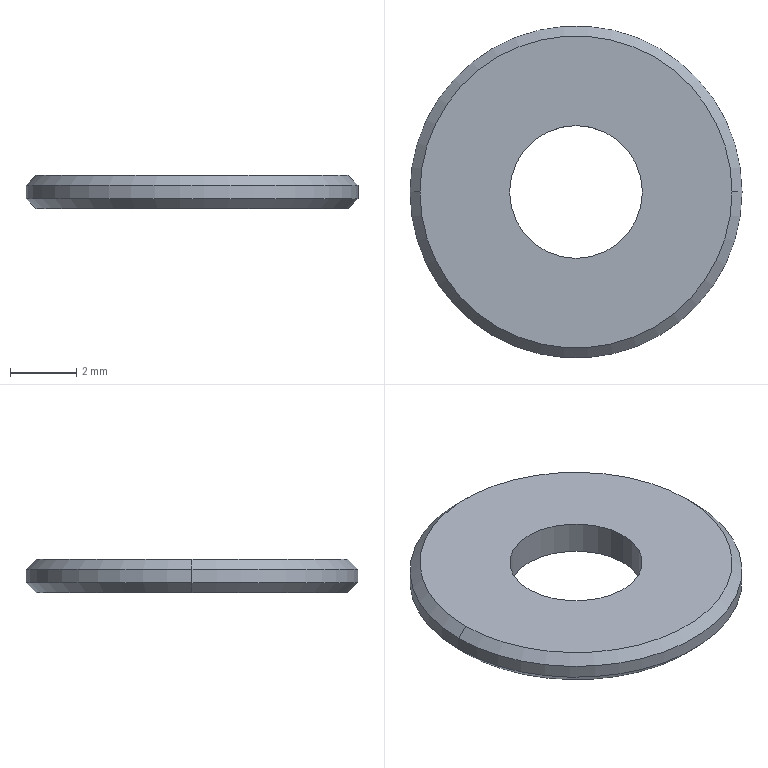Part | NX | features BREP 1 | 1 solid | 10 faces | box 10 x 10 x 1 mm | volume 63.203 mm3 | cone 4 | cylinder 4 | plane 2 | commonest cylinder face diameters 4 x2 10 x2
STEP:
#1=CARTESIAN_POINT('',(39.473,-510.005,1.));
#2=VERTEX_POINT('',#1);
#3=CARTESIAN_POINT('',(30.073,-510.005,1.));
#4=VERTEX_POINT('',#3);
#5=CARTESIAN_POINT('',(34.773,-510.005,1.));
#6=DIRECTION('',(0.,0.,1.));
#7=DIRECTION('',(1.,0.,0.));
#8=AXIS2_PLACEMENT_3D('',#5,#6,#7);
#9=CIRCLE('',#8,4.7);
#10=EDGE_CURVE('',#2,#4,#9,.T.);
#11=ORIENTED_EDGE('',*,*,#10,.F.);
#12=CARTESIAN_POINT('',(39.773,-510.005,0.7));
#13=VERTEX_POINT('',#12);
#14=CARTESIAN_POINT('',(39.473,-510.005,1.));
#15=DIRECTION('',(0.7071,0.,-0.7071));
#16=VECTOR('',#15,1000.);
#17=LINE('',#14,#16);
#18=EDGE_CURVE('',#13,#2,#17,.F.);
#19=ORIENTED_EDGE('',*,*,#18,.F.);
#20=CARTESIAN_POINT('',(29.773,-510.005,0.7));
#21=VERTEX_POINT('',#20);
#22=CARTESIAN_POINT('',(34.773,-510.005,0.7));
#23=DIRECTION('',(0.,0.,-1.));
#24=DIRECTION('',(1.,0.,0.));
#25=AXIS2_PLACEMENT_3D('',#22,#23,#24);
#26=CIRCLE('',#25,5.);
#27=EDGE_CURVE('',#21,#13,#26,.T.);
#28=ORIENTED_EDGE('',*,*,#27,.F.);
#29=CARTESIAN_POINT('',(30.073,-510.005,1.));
#30=DIRECTION('',(-0.7071,0.,-0.7071));
#31=VECTOR('',#30,1000.);
#32=LINE('',#29,#31);
#33=EDGE_CURVE('',#21,#4,#32,.F.);
#34=ORIENTED_EDGE('',*,*,#33,.T.);
#35=EDGE_LOOP('',(#11,#19,#28,#34));
#36=FACE_BOUND('',#35,.T.);
#37=CARTESIAN_POINT('',(34.773,-510.005,1.));
#38=DIRECTION('',(0.,0.,-1.));
#39=DIRECTION('',(1.,0.,0.));
#40=AXIS2_PLACEMENT_3D('',#37,#38,#39);
#41=CONICAL_SURFACE('',#40,4.7,0.7854);
#42=ADVANCED_FACE('',(#36),#41,.T.);
#43=CARTESIAN_POINT('',(30.073,-510.005,0.));
#44=VERTEX_POINT('',#43);
#45=CARTESIAN_POINT('',(39.473,-510.005,0.));
#46=VERTEX_POINT('',#45);
#47=CARTESIAN_POINT('',(34.773,-510.005,0.));
#48=DIRECTION('',(0.,0.,-1.));
#49=DIRECTION('',(1.,0.,0.));
#50=AXIS2_PLACEMENT_3D('',#47,#48,#49);
#51=CIRCLE('',#50,4.7);
#52=EDGE_CURVE('',#44,#46,#51,.T.);
#53=ORIENTED_EDGE('',*,*,#52,.F.);
#54=CARTESIAN_POINT('',(29.773,-510.005,0.3));
#55=VERTEX_POINT('',#54);
#56=CARTESIAN_POINT('',(29.773,-510.005,0.3));
#57=DIRECTION('',(-0.7071,0.,0.7071));
#58=VECTOR('',#57,1000.);
#59=LINE('',#56,#58);
#60=EDGE_CURVE('',#44,#55,#59,.T.);
#61=ORIENTED_EDGE('',*,*,#60,.T.);
#62=CARTESIAN_POINT('',(39.773,-510.005,0.3));
#63=VERTEX_POINT('',#62);
#64=CARTESIAN_POINT('',(34.773,-510.005,0.3));
#65=DIRECTION('',(0.,0.,1.));
#66=DIRECTION('',(1.,0.,0.));
#67=AXIS2_PLACEMENT_3D('',#64,#65,#66);
#68=CIRCLE('',#67,5.);
#69=EDGE_CURVE('',#63,#55,#68,.T.);
#70=ORIENTED_EDGE('',*,*,#69,.F.);
#71=CARTESIAN_POINT('',(39.773,-510.005,0.3));
#72=DIRECTION('',(0.7071,0.,0.7071));
#73=VECTOR('',#72,1000.);
#74=LINE('',#71,#73);
#75=EDGE_CURVE('',#46,#63,#74,.T.);
#76=ORIENTED_EDGE('',*,*,#75,.F.);
#77=EDGE_LOOP('',(#53,#61,#70,#76));
#78=FACE_BOUND('',#77,.T.);
#79=CARTESIAN_POINT('',(34.773,-510.005,0.3));
#80=DIRECTION('',(0.,0.,1.));
#81=DIRECTION('',(-1.,0.,0.));
#82=AXIS2_PLACEMENT_3D('',#79,#80,#81);
#83=CONICAL_SURFACE('',#82,5.,0.7854);
#84=ADVANCED_FACE('',(#78),#83,.T.);
#85=CARTESIAN_POINT('',(32.773,-510.005,1.));
#86=VERTEX_POINT('',#85);
#87=CARTESIAN_POINT('',(36.773,-510.005,1.));
#88=VERTEX_POINT('',#87);
#89=CARTESIAN_POINT('',(34.773,-510.005,1.));
#90=DIRECTION('',(0.,0.,1.));
#91=DIRECTION('',(1.,0.,0.));
#92=AXIS2_PLACEMENT_3D('',#89,#90,#91);
#93=CIRCLE('',#92,2.);
#94=EDGE_CURVE('',#86,#88,#93,.T.);
#95=ORIENTED_EDGE('',*,*,#94,.T.);
#96=CARTESIAN_POINT('',(36.773,-510.005,0.));
#97=VERTEX_POINT('',#96);
#98=CARTESIAN_POINT('',(36.773,-510.005,1.));
#99=DIRECTION('',(0.,0.,-1.));
#100=VECTOR('',#99,1000.);
#101=LINE('',#98,#100);
#102=EDGE_CURVE('',#97,#88,#101,.F.);
#103=ORIENTED_EDGE('',*,*,#102,.F.);
#104=CARTESIAN_POINT('',(32.773,-510.005,0.));
#105=VERTEX_POINT('',#104);
#106=CARTESIAN_POINT('',(34.773,-510.005,0.));
#107=DIRECTION('',(0.,0.,1.));
#108=DIRECTION('',(1.,0.,0.));
#109=AXIS2_PLACEMENT_3D('',#106,#107,#108);
#110=CIRCLE('',#109,2.);
#111=EDGE_CURVE('',#105,#97,#110,.T.);
#112=ORIENTED_EDGE('',*,*,#111,.F.);
#113=CARTESIAN_POINT('',(32.773,-510.005,1.));
#114=DIRECTION('',(0.,0.,-1.));
#115=VECTOR('',#114,1000.);
#116=LINE('',#113,#115);
#117=EDGE_CURVE('',#105,#86,#116,.F.);
#118=ORIENTED_EDGE('',*,*,#117,.T.);
#119=EDGE_LOOP('',(#95,#103,#112,#118));
#120=FACE_BOUND('',#119,.T.);
#121=CARTESIAN_POINT('',(34.773,-510.005,1.));
#122=DIRECTION('',(0.,0.,-1.));
#123=DIRECTION('',(1.,0.,0.));
#124=AXIS2_PLACEMENT_3D('',#121,#122,#123);
#125=CYLINDRICAL_SURFACE('',#124,2.);
#126=ADVANCED_FACE('',(#120),#125,.F.);
#127=ORIENTED_EDGE('',*,*,#27,.T.);
#128=CARTESIAN_POINT('',(39.773,-510.005,1.));
#129=DIRECTION('',(0.,0.,-1.));
#130=VECTOR('',#129,1000.);
#131=LINE('',#128,#130);
#132=EDGE_CURVE('',#63,#13,#131,.F.);
#133=ORIENTED_EDGE('',*,*,#132,.F.);
#134=ORIENTED_EDGE('',*,*,#69,.T.);
#135=CARTESIAN_POINT('',(29.773,-510.005,1.));
#136=DIRECTION('',(0.,0.,-1.));
#137=VECTOR('',#136,1000.);
#138=LINE('',#135,#137);
#139=EDGE_CURVE('',#55,#21,#138,.F.);
#140=ORIENTED_EDGE('',*,*,#139,.T.);
#141=EDGE_LOOP('',(#127,#133,#134,#140));
#142=FACE_BOUND('',#141,.T.);
#143=CARTESIAN_POINT('',(34.773,-510.005,1.));
#144=DIRECTION('',(0.,0.,-1.));
#145=DIRECTION('',(1.,0.,0.));
#146=AXIS2_PLACEMENT_3D('',#143,#144,#145);
#147=CYLINDRICAL_SURFACE('',#146,5.);
#148=ADVANCED_FACE('',(#142),#147,.T.);
#149=CARTESIAN_POINT('',(34.773,-510.005,1.));
#150=DIRECTION('',(0.,0.,1.));
#151=DIRECTION('',(1.,0.,0.));
#152=AXIS2_PLACEMENT_3D('',#149,#150,#151);
#153=CIRCLE('',#152,4.7);
#154=EDGE_CURVE('',#4,#2,#153,.T.);
#155=ORIENTED_EDGE('',*,*,#154,.T.);
#156=ORIENTED_EDGE('',*,*,#10,.T.);
#157=EDGE_LOOP('',(#155,#156));
#158=FACE_BOUND('',#157,.T.);
#159=ORIENTED_EDGE('',*,*,#94,.F.);
#160=CARTESIAN_POINT('',(34.773,-510.005,1.));
#161=DIRECTION('',(0.,0.,1.));
#162=DIRECTION('',(1.,0.,0.));
#163=AXIS2_PLACEMENT_3D('',#160,#161,#162);
#164=CIRCLE('',#163,2.);
#165=EDGE_CURVE('',#88,#86,#164,.T.);
#166=ORIENTED_EDGE('',*,*,#165,.F.);
#167=EDGE_LOOP('',(#159,#166));
#168=FACE_BOUND('',#167,.T.);
#169=CARTESIAN_POINT('',(34.773,-510.005,1.));
#170=DIRECTION('',(0.,0.,1.));
#171=DIRECTION('',(-1.,0.,0.));
#172=AXIS2_PLACEMENT_3D('',#169,#170,#171);
#173=PLANE('',#172);
#174=ADVANCED_FACE('',(#158,#168),#173,.T.);
#175=CARTESIAN_POINT('',(34.773,-510.005,0.));
#176=DIRECTION('',(0.,0.,-1.));
#177=DIRECTION('',(1.,0.,0.));
#178=AXIS2_PLACEMENT_3D('',#175,#176,#177);
#179=CIRCLE('',#178,4.7);
#180=EDGE_CURVE('',#46,#44,#179,.T.);
#181=ORIENTED_EDGE('',*,*,#180,.T.);
#182=ORIENTED_EDGE('',*,*,#52,.T.);
#183=EDGE_LOOP('',(#181,#182));
#184=FACE_BOUND('',#183,.T.);
#185=ORIENTED_EDGE('',*,*,#111,.T.);
#186=CARTESIAN_POINT('',(34.773,-510.005,0.));
#187=DIRECTION('',(0.,0.,1.));
#188=DIRECTION('',(1.,0.,0.));
#189=AXIS2_PLACEMENT_3D('',#186,#187,#188);
#190=CIRCLE('',#189,2.);
#191=EDGE_CURVE('',#97,#105,#190,.T.);
#192=ORIENTED_EDGE('',*,*,#191,.T.);
#193=EDGE_LOOP('',(#185,#192));
#194=FACE_BOUND('',#193,.T.);
#195=CARTESIAN_POINT('',(34.773,-510.005,0.));
#196=DIRECTION('',(0.,0.,1.));
#197=DIRECTION('',(-1.,0.,0.));
#198=AXIS2_PLACEMENT_3D('',#195,#196,#197);
#199=PLANE('',#198);
#200=ADVANCED_FACE('',(#184,#194),#199,.F.);
#201=ORIENTED_EDGE('',*,*,#132,.T.);
#202=CARTESIAN_POINT('',(34.773,-510.005,0.7));
#203=DIRECTION('',(0.,0.,-1.));
#204=DIRECTION('',(1.,0.,0.));
#205=AXIS2_PLACEMENT_3D('',#202,#203,#204);
#206=CIRCLE('',#205,5.);
#207=EDGE_CURVE('',#13,#21,#206,.T.);
#208=ORIENTED_EDGE('',*,*,#207,.T.);
#209=ORIENTED_EDGE('',*,*,#139,.F.);
#210=CARTESIAN_POINT('',(34.773,-510.005,0.3));
#211=DIRECTION('',(0.,0.,1.));
#212=DIRECTION('',(1.,0.,0.));
#213=AXIS2_PLACEMENT_3D('',#210,#211,#212);
#214=CIRCLE('',#213,5.);
#215=EDGE_CURVE('',#55,#63,#214,.T.);
#216=ORIENTED_EDGE('',*,*,#215,.T.);
#217=EDGE_LOOP('',(#201,#208,#209,#216));
#218=FACE_BOUND('',#217,.T.);
#219=CARTESIAN_POINT('',(34.773,-510.005,1.));
#220=DIRECTION('',(0.,0.,-1.));
#221=DIRECTION('',(1.,0.,0.));
#222=AXIS2_PLACEMENT_3D('',#219,#220,#221);
#223=CYLINDRICAL_SURFACE('',#222,5.);
#224=ADVANCED_FACE('',(#218),#223,.T.);
#225=ORIENTED_EDGE('',*,*,#102,.T.);
#226=ORIENTED_EDGE('',*,*,#165,.T.);
#227=ORIENTED_EDGE('',*,*,#117,.F.);
#228=ORIENTED_EDGE('',*,*,#191,.F.);
#229=EDGE_LOOP('',(#225,#226,#227,#228));
#230=FACE_BOUND('',#229,.T.);
#231=CARTESIAN_POINT('',(34.773,-510.005,1.));
#232=DIRECTION('',(0.,0.,-1.));
#233=DIRECTION('',(1.,0.,0.));
#234=AXIS2_PLACEMENT_3D('',#231,#232,#233);
#235=CYLINDRICAL_SURFACE('',#234,2.);
#236=ADVANCED_FACE('',(#230),#235,.F.);
#237=ORIENTED_EDGE('',*,*,#60,.F.);
#238=ORIENTED_EDGE('',*,*,#180,.F.);
#239=ORIENTED_EDGE('',*,*,#75,.T.);
#240=ORIENTED_EDGE('',*,*,#215,.F.);
#241=EDGE_LOOP('',(#237,#238,#239,#240));
#242=FACE_BOUND('',#241,.T.);
#243=CARTESIAN_POINT('',(34.773,-510.005,0.3));
#244=DIRECTION('',(0.,0.,1.));
#245=DIRECTION('',(-1.,0.,0.));
#246=AXIS2_PLACEMENT_3D('',#243,#244,#245);
#247=CONICAL_SURFACE('',#246,5.,0.7854);
#248=ADVANCED_FACE('',(#242),#247,.T.);
#249=ORIENTED_EDGE('',*,*,#18,.T.);
#250=ORIENTED_EDGE('',*,*,#154,.F.);
#251=ORIENTED_EDGE('',*,*,#33,.F.);
#252=ORIENTED_EDGE('',*,*,#207,.F.);
#253=EDGE_LOOP('',(#249,#250,#251,#252));
#254=FACE_BOUND('',#253,.T.);
#255=CARTESIAN_POINT('',(34.773,-510.005,1.));
#256=DIRECTION('',(0.,0.,-1.));
#257=DIRECTION('',(1.,0.,0.));
#258=AXIS2_PLACEMENT_3D('',#255,#256,#257);
#259=CONICAL_SURFACE('',#258,4.7,0.7854);
#260=ADVANCED_FACE('',(#254),#259,.T.);
#261=CLOSED_SHELL('',(#42,#84,#126,#148,#174,#200,#224,#236,#248,#260));
#262=MANIFOLD_SOLID_BREP('',#261);
#263=(LENGTH_UNIT()NAMED_UNIT(*)SI_UNIT(.MILLI.,.METRE.));
#264=UNCERTAINTY_MEASURE_WITH_UNIT(LENGTH_MEASURE(0.00001),#263,'','');
#265=(NAMED_UNIT(*)PLANE_ANGLE_UNIT()SI_UNIT($,.RADIAN.));
#266=(NAMED_UNIT(*)SI_UNIT($,.STERADIAN.)SOLID_ANGLE_UNIT());
#267=(GEOMETRIC_REPRESENTATION_CONTEXT(3)GLOBAL_UNCERTAINTY_ASSIGNED_CONTEXT((#264))GLOBAL_UNIT_ASSIGNED_CONTEXT((#263,#265,#266))REPRESENTATION_CONTEXT('',''));
#268=ADVANCED_BREP_SHAPE_REPRESENTATION('',(#262),#267);